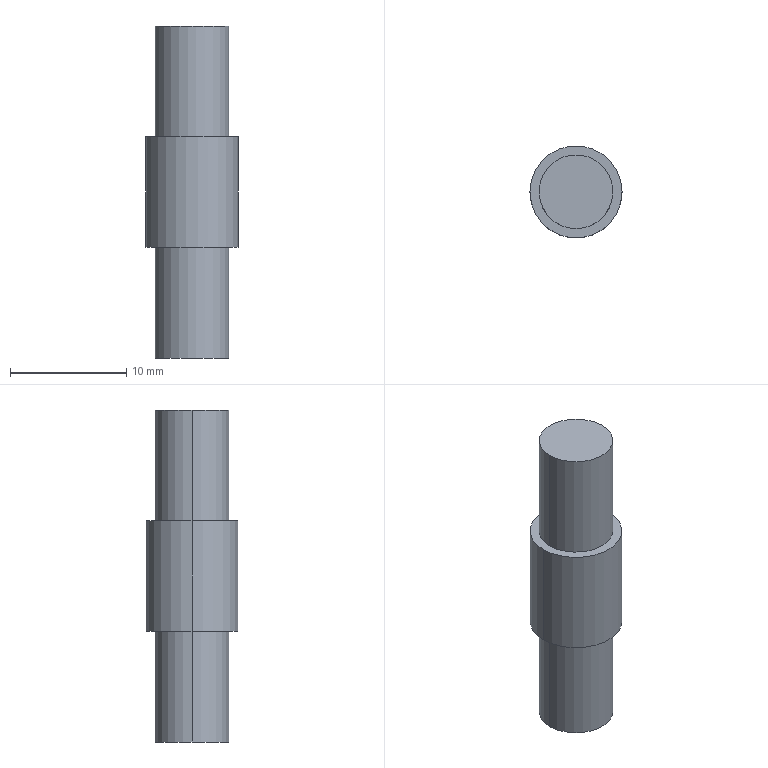Part | SolidWorks | features Extrusion 1, ICE 1 | 1 solid | 10 faces | box 7.925 x 7.925 x 28.575 mm | volume 1073 mm3 | cylinder 6 | plane 4 | commonest cylinder face diameters 6.35 x4 7.925 x2
STEP:
#1=CARTESIAN_POINT('',(3.175,0.,-14.287));
#2=VERTEX_POINT('',#1);
#3=CARTESIAN_POINT('',(-3.175,0.,-14.287));
#4=VERTEX_POINT('',#3);
#5=CARTESIAN_POINT('',(0.,0.,-14.287));
#6=DIRECTION('',(0.,0.,1.));
#7=DIRECTION('',(1.,0.,0.));
#8=AXIS2_PLACEMENT_3D('',#5,#6,#7);
#9=CIRCLE('',#8,3.175);
#10=EDGE_CURVE('',#2,#4,#9,.T.);
#11=ORIENTED_EDGE('',*,*,#10,.T.);
#12=CARTESIAN_POINT('',(-3.175,0.,-4.762));
#13=VERTEX_POINT('',#12);
#14=CARTESIAN_POINT('',(-3.175,0.,-14.287));
#15=DIRECTION('',(0.,0.,1.));
#16=VECTOR('',#15,1000.);
#17=LINE('',#14,#16);
#18=EDGE_CURVE('',#4,#13,#17,.T.);
#19=ORIENTED_EDGE('',*,*,#18,.T.);
#20=CARTESIAN_POINT('',(3.175,0.,-4.762));
#21=VERTEX_POINT('',#20);
#22=CARTESIAN_POINT('',(0.,0.,-4.762));
#23=DIRECTION('',(0.,0.,1.));
#24=DIRECTION('',(1.,0.,0.));
#25=AXIS2_PLACEMENT_3D('',#22,#23,#24);
#26=CIRCLE('',#25,3.175);
#27=EDGE_CURVE('',#21,#13,#26,.T.);
#28=ORIENTED_EDGE('',*,*,#27,.F.);
#29=CARTESIAN_POINT('',(3.175,0.,-14.287));
#30=DIRECTION('',(0.,0.,1.));
#31=VECTOR('',#30,1000.);
#32=LINE('',#29,#31);
#33=EDGE_CURVE('',#2,#21,#32,.T.);
#34=ORIENTED_EDGE('',*,*,#33,.F.);
#35=EDGE_LOOP('',(#11,#19,#28,#34));
#36=FACE_OUTER_BOUND('',#35,.T.);
#37=CARTESIAN_POINT('',(0.,0.,-14.287));
#38=DIRECTION('',(0.,0.,1.));
#39=DIRECTION('',(1.,0.,0.));
#40=AXIS2_PLACEMENT_3D('',#37,#38,#39);
#41=CYLINDRICAL_SURFACE('',#40,3.175);
#42=ADVANCED_FACE('',(#36),#41,.T.);
#43=CARTESIAN_POINT('',(3.175,0.,4.762));
#44=VERTEX_POINT('',#43);
#45=CARTESIAN_POINT('',(-3.175,0.,4.762));
#46=VERTEX_POINT('',#45);
#47=CARTESIAN_POINT('',(0.,0.,4.762));
#48=DIRECTION('',(0.,0.,1.));
#49=DIRECTION('',(1.,0.,0.));
#50=AXIS2_PLACEMENT_3D('',#47,#48,#49);
#51=CIRCLE('',#50,3.175);
#52=EDGE_CURVE('',#44,#46,#51,.T.);
#53=ORIENTED_EDGE('',*,*,#52,.T.);
#54=CARTESIAN_POINT('',(-3.175,0.,14.287));
#55=VERTEX_POINT('',#54);
#56=CARTESIAN_POINT('',(-3.175,0.,-14.287));
#57=DIRECTION('',(0.,0.,1.));
#58=VECTOR('',#57,1000.);
#59=LINE('',#56,#58);
#60=EDGE_CURVE('',#46,#55,#59,.T.);
#61=ORIENTED_EDGE('',*,*,#60,.T.);
#62=CARTESIAN_POINT('',(3.175,0.,14.287));
#63=VERTEX_POINT('',#62);
#64=CARTESIAN_POINT('',(0.,0.,14.287));
#65=DIRECTION('',(0.,0.,1.));
#66=DIRECTION('',(1.,0.,0.));
#67=AXIS2_PLACEMENT_3D('',#64,#65,#66);
#68=CIRCLE('',#67,3.175);
#69=EDGE_CURVE('',#63,#55,#68,.T.);
#70=ORIENTED_EDGE('',*,*,#69,.F.);
#71=CARTESIAN_POINT('',(3.175,0.,-14.287));
#72=DIRECTION('',(0.,0.,1.));
#73=VECTOR('',#72,1000.);
#74=LINE('',#71,#73);
#75=EDGE_CURVE('',#44,#63,#74,.T.);
#76=ORIENTED_EDGE('',*,*,#75,.F.);
#77=EDGE_LOOP('',(#53,#61,#70,#76));
#78=FACE_OUTER_BOUND('',#77,.T.);
#79=CARTESIAN_POINT('',(0.,0.,-14.287));
#80=DIRECTION('',(0.,0.,1.));
#81=DIRECTION('',(1.,0.,0.));
#82=AXIS2_PLACEMENT_3D('',#79,#80,#81);
#83=CYLINDRICAL_SURFACE('',#82,3.175);
#84=ADVANCED_FACE('',(#78),#83,.T.);
#85=CARTESIAN_POINT('',(3.962,0.,-4.762));
#86=VERTEX_POINT('',#85);
#87=CARTESIAN_POINT('',(-3.962,0.,-4.762));
#88=VERTEX_POINT('',#87);
#89=CARTESIAN_POINT('',(0.,0.,-4.762));
#90=DIRECTION('',(0.,0.,1.));
#91=DIRECTION('',(1.,0.,0.));
#92=AXIS2_PLACEMENT_3D('',#89,#90,#91);
#93=CIRCLE('',#92,3.962);
#94=EDGE_CURVE('',#86,#88,#93,.T.);
#95=ORIENTED_EDGE('',*,*,#94,.T.);
#96=CARTESIAN_POINT('',(-3.962,0.,4.762));
#97=VERTEX_POINT('',#96);
#98=CARTESIAN_POINT('',(-3.962,0.,-4.762));
#99=DIRECTION('',(0.,0.,1.));
#100=VECTOR('',#99,1000.);
#101=LINE('',#98,#100);
#102=EDGE_CURVE('',#88,#97,#101,.T.);
#103=ORIENTED_EDGE('',*,*,#102,.T.);
#104=CARTESIAN_POINT('',(3.962,0.,4.762));
#105=VERTEX_POINT('',#104);
#106=CARTESIAN_POINT('',(0.,0.,4.762));
#107=DIRECTION('',(0.,0.,1.));
#108=DIRECTION('',(1.,0.,0.));
#109=AXIS2_PLACEMENT_3D('',#106,#107,#108);
#110=CIRCLE('',#109,3.962);
#111=EDGE_CURVE('',#105,#97,#110,.T.);
#112=ORIENTED_EDGE('',*,*,#111,.F.);
#113=CARTESIAN_POINT('',(3.962,0.,-4.762));
#114=DIRECTION('',(0.,0.,1.));
#115=VECTOR('',#114,1000.);
#116=LINE('',#113,#115);
#117=EDGE_CURVE('',#86,#105,#116,.T.);
#118=ORIENTED_EDGE('',*,*,#117,.F.);
#119=EDGE_LOOP('',(#95,#103,#112,#118));
#120=FACE_OUTER_BOUND('',#119,.T.);
#121=CARTESIAN_POINT('',(0.,0.,-4.762));
#122=DIRECTION('',(0.,0.,1.));
#123=DIRECTION('',(1.,0.,0.));
#124=AXIS2_PLACEMENT_3D('',#121,#122,#123);
#125=CYLINDRICAL_SURFACE('',#124,3.962);
#126=ADVANCED_FACE('',(#120),#125,.T.);
#127=ORIENTED_EDGE('',*,*,#102,.F.);
#128=CARTESIAN_POINT('',(0.,0.,-4.762));
#129=DIRECTION('',(0.,0.,1.));
#130=DIRECTION('',(1.,0.,0.));
#131=AXIS2_PLACEMENT_3D('',#128,#129,#130);
#132=CIRCLE('',#131,3.962);
#133=EDGE_CURVE('',#88,#86,#132,.T.);
#134=ORIENTED_EDGE('',*,*,#133,.T.);
#135=ORIENTED_EDGE('',*,*,#117,.T.);
#136=CARTESIAN_POINT('',(0.,0.,4.762));
#137=DIRECTION('',(0.,0.,1.));
#138=DIRECTION('',(1.,0.,0.));
#139=AXIS2_PLACEMENT_3D('',#136,#137,#138);
#140=CIRCLE('',#139,3.962);
#141=EDGE_CURVE('',#97,#105,#140,.T.);
#142=ORIENTED_EDGE('',*,*,#141,.F.);
#143=EDGE_LOOP('',(#127,#134,#135,#142));
#144=FACE_OUTER_BOUND('',#143,.T.);
#145=CARTESIAN_POINT('',(0.,0.,-4.762));
#146=DIRECTION('',(0.,0.,1.));
#147=DIRECTION('',(1.,0.,0.));
#148=AXIS2_PLACEMENT_3D('',#145,#146,#147);
#149=CYLINDRICAL_SURFACE('',#148,3.962);
#150=ADVANCED_FACE('',(#144),#149,.T.);
#151=ORIENTED_EDGE('',*,*,#27,.T.);
#152=CARTESIAN_POINT('',(0.,0.,-4.762));
#153=DIRECTION('',(0.,0.,1.));
#154=DIRECTION('',(1.,0.,0.));
#155=AXIS2_PLACEMENT_3D('',#152,#153,#154);
#156=CIRCLE('',#155,3.175);
#157=EDGE_CURVE('',#13,#21,#156,.T.);
#158=ORIENTED_EDGE('',*,*,#157,.T.);
#159=EDGE_LOOP('',(#151,#158));
#160=FACE_BOUND('',#159,.T.);
#161=ORIENTED_EDGE('',*,*,#94,.F.);
#162=ORIENTED_EDGE('',*,*,#133,.F.);
#163=EDGE_LOOP('',(#161,#162));
#164=FACE_OUTER_BOUND('',#163,.T.);
#165=CARTESIAN_POINT('',(0.,0.,-4.762));
#166=DIRECTION('',(0.,0.,1.));
#167=DIRECTION('',(1.,0.,0.));
#168=AXIS2_PLACEMENT_3D('',#165,#166,#167);
#169=PLANE('',#168);
#170=ADVANCED_FACE('',(#160,#164),#169,.F.);
#171=ORIENTED_EDGE('',*,*,#52,.F.);
#172=CARTESIAN_POINT('',(0.,0.,4.762));
#173=DIRECTION('',(0.,0.,1.));
#174=DIRECTION('',(1.,0.,0.));
#175=AXIS2_PLACEMENT_3D('',#172,#173,#174);
#176=CIRCLE('',#175,3.175);
#177=EDGE_CURVE('',#46,#44,#176,.T.);
#178=ORIENTED_EDGE('',*,*,#177,.F.);
#179=EDGE_LOOP('',(#171,#178));
#180=FACE_BOUND('',#179,.T.);
#181=ORIENTED_EDGE('',*,*,#111,.T.);
#182=ORIENTED_EDGE('',*,*,#141,.T.);
#183=EDGE_LOOP('',(#181,#182));
#184=FACE_OUTER_BOUND('',#183,.T.);
#185=CARTESIAN_POINT('',(0.,0.,4.762));
#186=DIRECTION('',(0.,0.,1.));
#187=DIRECTION('',(1.,0.,0.));
#188=AXIS2_PLACEMENT_3D('',#185,#186,#187);
#189=PLANE('',#188);
#190=ADVANCED_FACE('',(#180,#184),#189,.T.);
#191=ORIENTED_EDGE('',*,*,#69,.T.);
#192=CARTESIAN_POINT('',(0.,0.,14.287));
#193=DIRECTION('',(0.,0.,1.));
#194=DIRECTION('',(1.,0.,0.));
#195=AXIS2_PLACEMENT_3D('',#192,#193,#194);
#196=CIRCLE('',#195,3.175);
#197=EDGE_CURVE('',#55,#63,#196,.T.);
#198=ORIENTED_EDGE('',*,*,#197,.T.);
#199=EDGE_LOOP('',(#191,#198));
#200=FACE_OUTER_BOUND('',#199,.T.);
#201=CARTESIAN_POINT('',(0.,0.,14.287));
#202=DIRECTION('',(0.,0.,1.));
#203=DIRECTION('',(1.,0.,0.));
#204=AXIS2_PLACEMENT_3D('',#201,#202,#203);
#205=PLANE('',#204);
#206=ADVANCED_FACE('',(#200),#205,.T.);
#207=ORIENTED_EDGE('',*,*,#60,.F.);
#208=ORIENTED_EDGE('',*,*,#177,.T.);
#209=ORIENTED_EDGE('',*,*,#75,.T.);
#210=ORIENTED_EDGE('',*,*,#197,.F.);
#211=EDGE_LOOP('',(#207,#208,#209,#210));
#212=FACE_OUTER_BOUND('',#211,.T.);
#213=CARTESIAN_POINT('',(0.,0.,-14.287));
#214=DIRECTION('',(0.,0.,1.));
#215=DIRECTION('',(1.,0.,0.));
#216=AXIS2_PLACEMENT_3D('',#213,#214,#215);
#217=CYLINDRICAL_SURFACE('',#216,3.175);
#218=ADVANCED_FACE('',(#212),#217,.T.);
#219=ORIENTED_EDGE('',*,*,#18,.F.);
#220=CARTESIAN_POINT('',(0.,0.,-14.287));
#221=DIRECTION('',(0.,0.,1.));
#222=DIRECTION('',(1.,0.,0.));
#223=AXIS2_PLACEMENT_3D('',#220,#221,#222);
#224=CIRCLE('',#223,3.175);
#225=EDGE_CURVE('',#4,#2,#224,.T.);
#226=ORIENTED_EDGE('',*,*,#225,.T.);
#227=ORIENTED_EDGE('',*,*,#33,.T.);
#228=ORIENTED_EDGE('',*,*,#157,.F.);
#229=EDGE_LOOP('',(#219,#226,#227,#228));
#230=FACE_OUTER_BOUND('',#229,.T.);
#231=CARTESIAN_POINT('',(0.,0.,-14.287));
#232=DIRECTION('',(0.,0.,1.));
#233=DIRECTION('',(1.,0.,0.));
#234=AXIS2_PLACEMENT_3D('',#231,#232,#233);
#235=CYLINDRICAL_SURFACE('',#234,3.175);
#236=ADVANCED_FACE('',(#230),#235,.T.);
#237=ORIENTED_EDGE('',*,*,#10,.F.);
#238=ORIENTED_EDGE('',*,*,#225,.F.);
#239=EDGE_LOOP('',(#237,#238));
#240=FACE_OUTER_BOUND('',#239,.T.);
#241=CARTESIAN_POINT('',(0.,0.,-14.287));
#242=DIRECTION('',(0.,0.,1.));
#243=DIRECTION('',(1.,0.,0.));
#244=AXIS2_PLACEMENT_3D('',#241,#242,#243);
#245=PLANE('',#244);
#246=ADVANCED_FACE('',(#240),#245,.F.);
#247=CLOSED_SHELL('',(#42,#84,#126,#150,#170,#190,#206,#218,#236,#246));
#248=MANIFOLD_SOLID_BREP('',#247);
#249=CARTESIAN_POINT('',(0.,0.,0.));
#250=DIRECTION('',(0.,0.,1.));
#251=DIRECTION('',(1.,0.,0.));
#252=AXIS2_PLACEMENT_3D('',#249,#250,#251);
#253=(LENGTH_UNIT()NAMED_UNIT(*)SI_UNIT(.MILLI.,.METRE.));
#254=UNCERTAINTY_MEASURE_WITH_UNIT(LENGTH_MEASURE(0.00001),#253,'','');
#255=(NAMED_UNIT(*)PLANE_ANGLE_UNIT()SI_UNIT($,.RADIAN.));
#256=(NAMED_UNIT(*)SI_UNIT($,.STERADIAN.)SOLID_ANGLE_UNIT());
#257=(GEOMETRIC_REPRESENTATION_CONTEXT(3)GLOBAL_UNCERTAINTY_ASSIGNED_CONTEXT((#254))GLOBAL_UNIT_ASSIGNED_CONTEXT((#253,#255,#256))REPRESENTATION_CONTEXT('',''));
#258=ADVANCED_BREP_SHAPE_REPRESENTATION('',(#248,#252),#257);